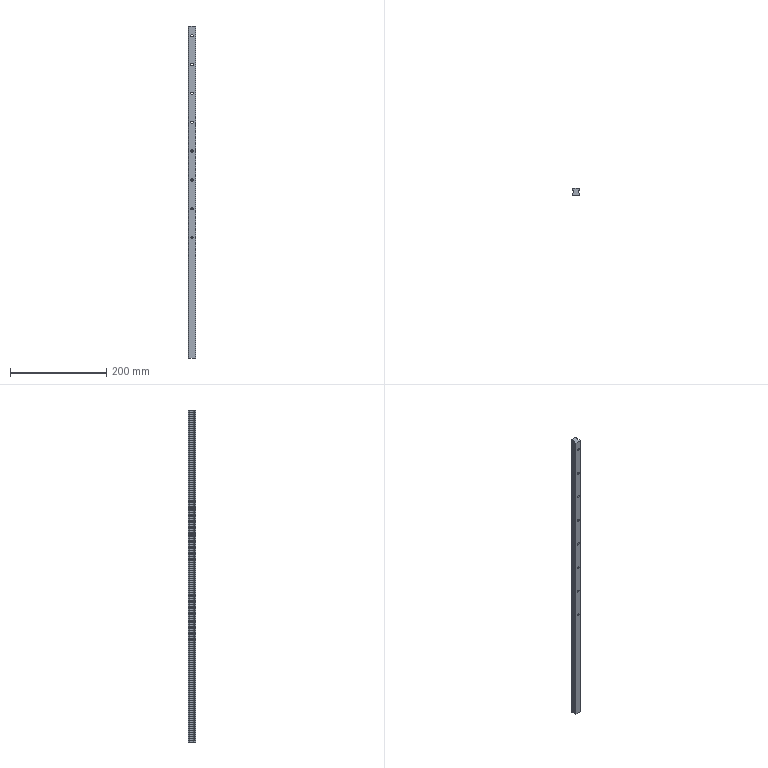Part | STEP file | ASND-0110-HGR15_1_1 | 1 solid | 76 faces | box 15 x 15 x 690 mm | volume 128296 mm3 | cylinder 46 | plane 30 | commonest cylinder face diameters 7.5 x16 5.102 x10 0.8 x8 4.5 x6 3.24 x4 2 x2